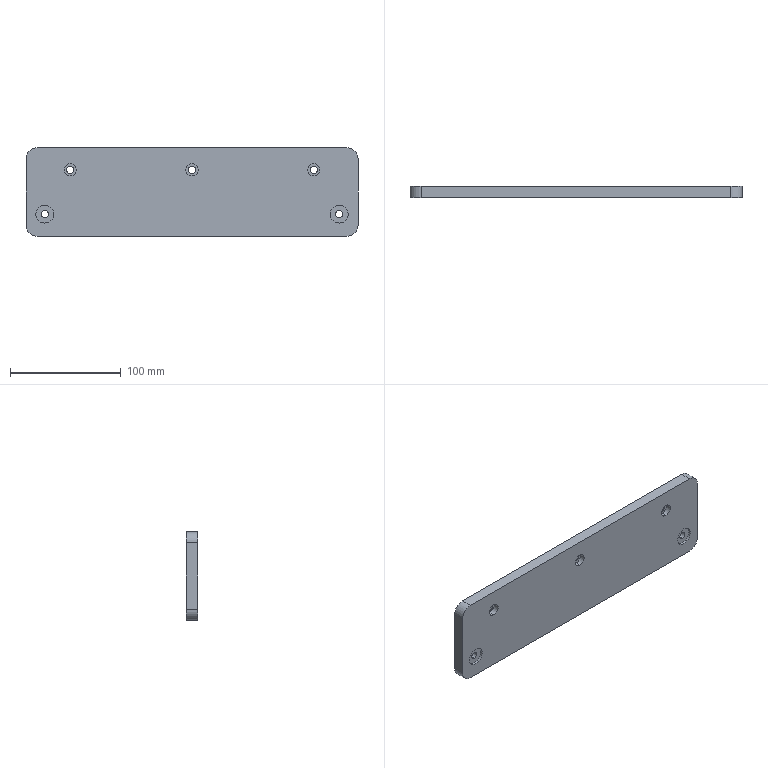Part | STEP file | PN_0028 | 1 solid | 35 faces | box 300 x 10 x 80 mm | volume 235858 mm3 | cylinder 24 | plane 11 | commonest cylinder face diameters 6.6 x6 11 x6 6.5 x4 16.1 x4 20 x4